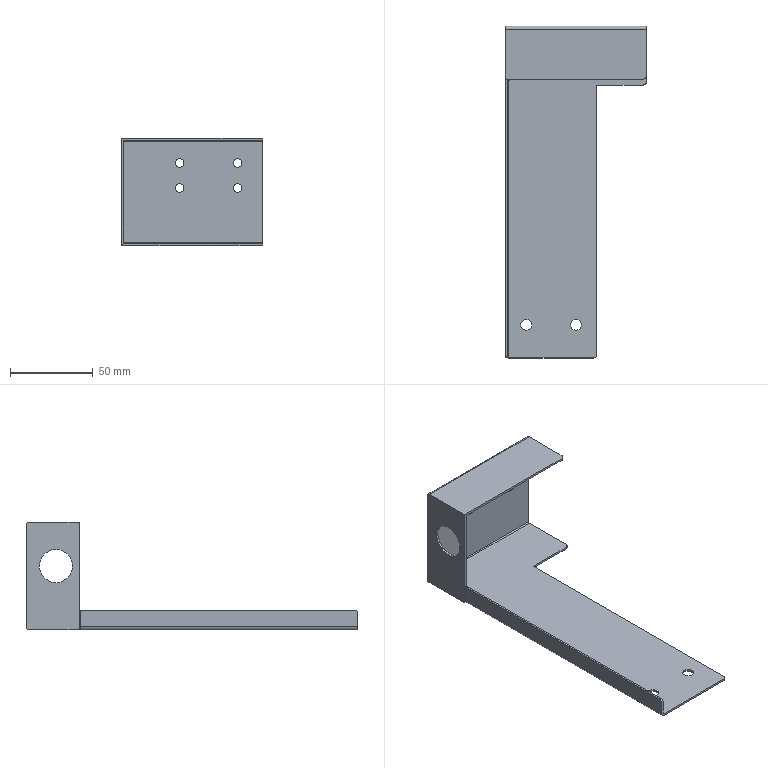Part | 1 solid | 50 faces | box 85 x 200 x 65 mm | volume 27815 mm3 | plane 26 | cylinder 24 | commonest cylinder face diameters 5.2 x8 4 x4 6.5 x4 1.473 x3 3.873 x3 20 x2
STEP:
#1=CARTESIAN_POINT('',(-26.3,82.,47.3));
#2=VERTEX_POINT('',#1);
#3=CARTESIAN_POINT('',(-26.3,82.,27.3));
#4=VERTEX_POINT('',#3);
#5=CARTESIAN_POINT('',(-26.3,82.,37.3));
#6=DIRECTION('',(1.,0.,0.));
#7=DIRECTION('',(0.,0.,-1.));
#8=AXIS2_PLACEMENT_3D('',#5,#6,#7);
#9=CIRCLE('',#8,10.);
#10=EDGE_CURVE('',#2,#4,#9,.T.);
#11=ORIENTED_EDGE('',*,*,#10,.T.);
#12=CARTESIAN_POINT('',(-27.5,82.,27.3));
#13=VERTEX_POINT('',#12);
#14=CARTESIAN_POINT('',(57.5,82.,27.3));
#15=DIRECTION('',(-1.,0.,0.));
#16=VECTOR('',#15,1000.);
#17=LINE('',#14,#16);
#18=EDGE_CURVE('',#4,#13,#17,.T.);
#19=ORIENTED_EDGE('',*,*,#18,.T.);
#20=CARTESIAN_POINT('',(-27.5,82.,47.3));
#21=VERTEX_POINT('',#20);
#22=CARTESIAN_POINT('',(-27.5,82.,37.3));
#23=DIRECTION('',(-1.,0.,0.));
#24=DIRECTION('',(0.,0.,1.));
#25=AXIS2_PLACEMENT_3D('',#22,#23,#24);
#26=CIRCLE('',#25,10.);
#27=EDGE_CURVE('',#13,#21,#26,.T.);
#28=ORIENTED_EDGE('',*,*,#27,.T.);
#29=CARTESIAN_POINT('',(57.5,82.,47.3));
#30=DIRECTION('',(-1.,0.,0.));
#31=VECTOR('',#30,1000.);
#32=LINE('',#29,#31);
#33=EDGE_CURVE('',#2,#21,#32,.T.);
#34=ORIENTED_EDGE('',*,*,#33,.F.);
#35=EDGE_LOOP('',(#11,#19,#28,#34));
#36=FACE_OUTER_BOUND('',#35,.T.);
#37=CARTESIAN_POINT('',(57.5,82.,37.3));
#38=DIRECTION('',(-1.,0.,0.));
#39=DIRECTION('',(0.,0.,1.));
#40=AXIS2_PLACEMENT_3D('',#37,#38,#39);
#41=CYLINDRICAL_SURFACE('',#40,10.);
#42=ADVANCED_FACE('',(#36),#41,.F.);
#43=CARTESIAN_POINT('',(42.5,98.8,46.2));
#44=VERTEX_POINT('',#43);
#45=CARTESIAN_POINT('',(42.5,98.8,51.4));
#46=VERTEX_POINT('',#45);
#47=CARTESIAN_POINT('',(42.5,98.8,48.8));
#48=DIRECTION('',(0.,1.,0.));
#49=DIRECTION('',(0.,0.,1.));
#50=AXIS2_PLACEMENT_3D('',#47,#48,#49);
#51=CIRCLE('',#50,2.6);
#52=EDGE_CURVE('',#44,#46,#51,.T.);
#53=ORIENTED_EDGE('',*,*,#52,.F.);
#54=CARTESIAN_POINT('',(42.5,100.,46.2));
#55=VERTEX_POINT('',#54);
#56=CARTESIAN_POINT('',(42.5,90.,46.2));
#57=DIRECTION('',(0.,1.,0.));
#58=VECTOR('',#57,1000.);
#59=LINE('',#56,#58);
#60=EDGE_CURVE('',#44,#55,#59,.T.);
#61=ORIENTED_EDGE('',*,*,#60,.T.);
#62=CARTESIAN_POINT('',(42.5,100.,51.4));
#63=VERTEX_POINT('',#62);
#64=CARTESIAN_POINT('',(42.5,100.,48.8));
#65=DIRECTION('',(0.,1.,0.));
#66=DIRECTION('',(0.,0.,1.));
#67=AXIS2_PLACEMENT_3D('',#64,#65,#66);
#68=CIRCLE('',#67,2.6);
#69=EDGE_CURVE('',#55,#63,#68,.T.);
#70=ORIENTED_EDGE('',*,*,#69,.T.);
#71=CARTESIAN_POINT('',(42.5,90.,51.4));
#72=DIRECTION('',(0.,1.,0.));
#73=VECTOR('',#72,1000.);
#74=LINE('',#71,#73);
#75=EDGE_CURVE('',#46,#63,#74,.T.);
#76=ORIENTED_EDGE('',*,*,#75,.F.);
#77=EDGE_LOOP('',(#53,#61,#70,#76));
#78=FACE_OUTER_BOUND('',#77,.T.);
#79=CARTESIAN_POINT('',(42.5,90.,48.8));
#80=DIRECTION('',(0.,1.,0.));
#81=DIRECTION('',(0.,0.,1.));
#82=AXIS2_PLACEMENT_3D('',#79,#80,#81);
#83=CYLINDRICAL_SURFACE('',#82,2.6);
#84=ADVANCED_FACE('',(#78),#83,.F.);
#85=CARTESIAN_POINT('',(7.5,98.8,46.2));
#86=VERTEX_POINT('',#85);
#87=CARTESIAN_POINT('',(7.5,98.8,51.4));
#88=VERTEX_POINT('',#87);
#89=CARTESIAN_POINT('',(7.5,98.8,48.8));
#90=DIRECTION('',(0.,1.,0.));
#91=DIRECTION('',(0.,0.,1.));
#92=AXIS2_PLACEMENT_3D('',#89,#90,#91);
#93=CIRCLE('',#92,2.6);
#94=EDGE_CURVE('',#86,#88,#93,.T.);
#95=ORIENTED_EDGE('',*,*,#94,.F.);
#96=CARTESIAN_POINT('',(7.5,100.,46.2));
#97=VERTEX_POINT('',#96);
#98=CARTESIAN_POINT('',(7.5,90.,46.2));
#99=DIRECTION('',(0.,1.,0.));
#100=VECTOR('',#99,1000.);
#101=LINE('',#98,#100);
#102=EDGE_CURVE('',#86,#97,#101,.T.);
#103=ORIENTED_EDGE('',*,*,#102,.T.);
#104=CARTESIAN_POINT('',(7.5,100.,51.4));
#105=VERTEX_POINT('',#104);
#106=CARTESIAN_POINT('',(7.5,100.,48.8));
#107=DIRECTION('',(0.,1.,0.));
#108=DIRECTION('',(0.,0.,1.));
#109=AXIS2_PLACEMENT_3D('',#106,#107,#108);
#110=CIRCLE('',#109,2.6);
#111=EDGE_CURVE('',#97,#105,#110,.T.);
#112=ORIENTED_EDGE('',*,*,#111,.T.);
#113=CARTESIAN_POINT('',(7.5,90.,51.4));
#114=DIRECTION('',(0.,1.,0.));
#115=VECTOR('',#114,1000.);
#116=LINE('',#113,#115);
#117=EDGE_CURVE('',#88,#105,#116,.T.);
#118=ORIENTED_EDGE('',*,*,#117,.F.);
#119=EDGE_LOOP('',(#95,#103,#112,#118));
#120=FACE_OUTER_BOUND('',#119,.T.);
#121=CARTESIAN_POINT('',(7.5,90.,48.8));
#122=DIRECTION('',(0.,1.,0.));
#123=DIRECTION('',(0.,0.,1.));
#124=AXIS2_PLACEMENT_3D('',#121,#122,#123);
#125=CYLINDRICAL_SURFACE('',#124,2.6);
#126=ADVANCED_FACE('',(#120),#125,.F.);
#127=CARTESIAN_POINT('',(7.5,98.8,31.2));
#128=VERTEX_POINT('',#127);
#129=CARTESIAN_POINT('',(7.5,98.8,36.4));
#130=VERTEX_POINT('',#129);
#131=CARTESIAN_POINT('',(7.5,98.8,33.8));
#132=DIRECTION('',(0.,1.,0.));
#133=DIRECTION('',(0.,0.,1.));
#134=AXIS2_PLACEMENT_3D('',#131,#132,#133);
#135=CIRCLE('',#134,2.6);
#136=EDGE_CURVE('',#128,#130,#135,.T.);
#137=ORIENTED_EDGE('',*,*,#136,.F.);
#138=CARTESIAN_POINT('',(7.5,100.,31.2));
#139=VERTEX_POINT('',#138);
#140=CARTESIAN_POINT('',(7.5,90.,31.2));
#141=DIRECTION('',(0.,1.,0.));
#142=VECTOR('',#141,1000.);
#143=LINE('',#140,#142);
#144=EDGE_CURVE('',#128,#139,#143,.T.);
#145=ORIENTED_EDGE('',*,*,#144,.T.);
#146=CARTESIAN_POINT('',(7.5,100.,36.4));
#147=VERTEX_POINT('',#146);
#148=CARTESIAN_POINT('',(7.5,100.,33.8));
#149=DIRECTION('',(0.,1.,0.));
#150=DIRECTION('',(0.,0.,1.));
#151=AXIS2_PLACEMENT_3D('',#148,#149,#150);
#152=CIRCLE('',#151,2.6);
#153=EDGE_CURVE('',#139,#147,#152,.T.);
#154=ORIENTED_EDGE('',*,*,#153,.T.);
#155=CARTESIAN_POINT('',(7.5,90.,36.4));
#156=DIRECTION('',(0.,1.,0.));
#157=VECTOR('',#156,1000.);
#158=LINE('',#155,#157);
#159=EDGE_CURVE('',#130,#147,#158,.T.);
#160=ORIENTED_EDGE('',*,*,#159,.F.);
#161=EDGE_LOOP('',(#137,#145,#154,#160));
#162=FACE_OUTER_BOUND('',#161,.T.);
#163=CARTESIAN_POINT('',(7.5,90.,33.8));
#164=DIRECTION('',(0.,1.,0.));
#165=DIRECTION('',(0.,0.,1.));
#166=AXIS2_PLACEMENT_3D('',#163,#164,#165);
#167=CYLINDRICAL_SURFACE('',#166,2.6);
#168=ADVANCED_FACE('',(#162),#167,.F.);
#169=CARTESIAN_POINT('',(42.5,98.8,31.2));
#170=VERTEX_POINT('',#169);
#171=CARTESIAN_POINT('',(42.5,98.8,36.4));
#172=VERTEX_POINT('',#171);
#173=CARTESIAN_POINT('',(42.5,98.8,33.8));
#174=DIRECTION('',(0.,1.,0.));
#175=DIRECTION('',(0.,0.,1.));
#176=AXIS2_PLACEMENT_3D('',#173,#174,#175);
#177=CIRCLE('',#176,2.6);
#178=EDGE_CURVE('',#170,#172,#177,.T.);
#179=ORIENTED_EDGE('',*,*,#178,.F.);
#180=CARTESIAN_POINT('',(42.5,100.,31.2));
#181=VERTEX_POINT('',#180);
#182=CARTESIAN_POINT('',(42.5,90.,31.2));
#183=DIRECTION('',(0.,1.,0.));
#184=VECTOR('',#183,1000.);
#185=LINE('',#182,#184);
#186=EDGE_CURVE('',#170,#181,#185,.T.);
#187=ORIENTED_EDGE('',*,*,#186,.T.);
#188=CARTESIAN_POINT('',(42.5,100.,36.4));
#189=VERTEX_POINT('',#188);
#190=CARTESIAN_POINT('',(42.5,100.,33.8));
#191=DIRECTION('',(0.,1.,0.));
#192=DIRECTION('',(0.,0.,1.));
#193=AXIS2_PLACEMENT_3D('',#190,#191,#192);
#194=CIRCLE('',#193,2.6);
#195=EDGE_CURVE('',#181,#189,#194,.T.);
#196=ORIENTED_EDGE('',*,*,#195,.T.);
#197=CARTESIAN_POINT('',(42.5,90.,36.4));
#198=DIRECTION('',(0.,1.,0.));
#199=VECTOR('',#198,1000.);
#200=LINE('',#197,#199);
#201=EDGE_CURVE('',#172,#189,#200,.T.);
#202=ORIENTED_EDGE('',*,*,#201,.F.);
#203=EDGE_LOOP('',(#179,#187,#196,#202));
#204=FACE_OUTER_BOUND('',#203,.T.);
#205=CARTESIAN_POINT('',(42.5,90.,33.8));
#206=DIRECTION('',(0.,1.,0.));
#207=DIRECTION('',(0.,0.,1.));
#208=AXIS2_PLACEMENT_3D('',#205,#206,#207);
#209=CYLINDRICAL_SURFACE('',#208,2.6);
#210=ADVANCED_FACE('',(#204),#209,.F.);
#211=CARTESIAN_POINT('',(18.25,-80.,0.));
#212=VERTEX_POINT('',#211);
#213=CARTESIAN_POINT('',(11.75,-80.,0.));
#214=VERTEX_POINT('',#213);
#215=CARTESIAN_POINT('',(15.,-80.,0.));
#216=DIRECTION('',(0.,0.,-1.));
#217=DIRECTION('',(-1.,0.,0.));
#218=AXIS2_PLACEMENT_3D('',#215,#216,#217);
#219=CIRCLE('',#218,3.25);
#220=EDGE_CURVE('',#212,#214,#219,.T.);
#221=ORIENTED_EDGE('',*,*,#220,.F.);
#222=CARTESIAN_POINT('',(18.25,-80.,-1.2));
#223=VERTEX_POINT('',#222);
#224=CARTESIAN_POINT('',(18.25,-80.,8.8));
#225=DIRECTION('',(0.,0.,-1.));
#226=VECTOR('',#225,1000.);
#227=LINE('',#224,#226);
#228=EDGE_CURVE('',#212,#223,#227,.T.);
#229=ORIENTED_EDGE('',*,*,#228,.T.);
#230=CARTESIAN_POINT('',(11.75,-80.,-1.2));
#231=VERTEX_POINT('',#230);
#232=CARTESIAN_POINT('',(15.,-80.,-1.2));
#233=DIRECTION('',(0.,0.,-1.));
#234=DIRECTION('',(-1.,0.,0.));
#235=AXIS2_PLACEMENT_3D('',#232,#233,#234);
#236=CIRCLE('',#235,3.25);
#237=EDGE_CURVE('',#223,#231,#236,.T.);
#238=ORIENTED_EDGE('',*,*,#237,.T.);
#239=CARTESIAN_POINT('',(11.75,-80.,8.8));
#240=DIRECTION('',(0.,0.,-1.));
#241=VECTOR('',#240,1000.);
#242=LINE('',#239,#241);
#243=EDGE_CURVE('',#214,#231,#242,.T.);
#244=ORIENTED_EDGE('',*,*,#243,.F.);
#245=EDGE_LOOP('',(#221,#229,#238,#244));
#246=FACE_OUTER_BOUND('',#245,.T.);
#247=CARTESIAN_POINT('',(15.,-80.,8.8));
#248=DIRECTION('',(0.,0.,-1.));
#249=DIRECTION('',(-1.,0.,0.));
#250=AXIS2_PLACEMENT_3D('',#247,#248,#249);
#251=CYLINDRICAL_SURFACE('',#250,3.25);
#252=ADVANCED_FACE('',(#246),#251,.F.);
#253=CARTESIAN_POINT('',(-11.75,-80.,0.));
#254=VERTEX_POINT('',#253);
#255=CARTESIAN_POINT('',(-18.25,-80.,0.));
#256=VERTEX_POINT('',#255);
#257=CARTESIAN_POINT('',(-15.,-80.,0.));
#258=DIRECTION('',(0.,0.,-1.));
#259=DIRECTION('',(-1.,0.,0.));
#260=AXIS2_PLACEMENT_3D('',#257,#258,#259);
#261=CIRCLE('',#260,3.25);
#262=EDGE_CURVE('',#254,#256,#261,.T.);
#263=ORIENTED_EDGE('',*,*,#262,.F.);
#264=CARTESIAN_POINT('',(-11.75,-80.,-1.2));
#265=VERTEX_POINT('',#264);
#266=CARTESIAN_POINT('',(-11.75,-80.,8.8));
#267=DIRECTION('',(0.,0.,-1.));
#268=VECTOR('',#267,1000.);
#269=LINE('',#266,#268);
#270=EDGE_CURVE('',#254,#265,#269,.T.);
#271=ORIENTED_EDGE('',*,*,#270,.T.);
#272=CARTESIAN_POINT('',(-18.25,-80.,-1.2));
#273=VERTEX_POINT('',#272);
#274=CARTESIAN_POINT('',(-15.,-80.,-1.2));
#275=DIRECTION('',(0.,0.,-1.));
#276=DIRECTION('',(-1.,0.,0.));
#277=AXIS2_PLACEMENT_3D('',#274,#275,#276);
#278=CIRCLE('',#277,3.25);
#279=EDGE_CURVE('',#265,#273,#278,.T.);
#280=ORIENTED_EDGE('',*,*,#279,.T.);
#281=CARTESIAN_POINT('',(-18.25,-80.,8.8));
#282=DIRECTION('',(0.,0.,-1.));
#283=VECTOR('',#282,1000.);
#284=LINE('',#281,#283);
#285=EDGE_CURVE('',#256,#273,#284,.T.);
#286=ORIENTED_EDGE('',*,*,#285,.F.);
#287=EDGE_LOOP('',(#263,#271,#280,#286));
#288=FACE_OUTER_BOUND('',#287,.T.);
#289=CARTESIAN_POINT('',(-15.,-80.,8.8));
#290=DIRECTION('',(0.,0.,-1.));
#291=DIRECTION('',(-1.,0.,0.));
#292=AXIS2_PLACEMENT_3D('',#289,#290,#291);
#293=CYLINDRICAL_SURFACE('',#292,3.25);
#294=ADVANCED_FACE('',(#288),#293,.F.);
#295=CARTESIAN_POINT('',(27.5,64.5,-1.2));
#296=VERTEX_POINT('',#295);
#297=CARTESIAN_POINT('',(27.5,-98.,-1.2));
#298=VERTEX_POINT('',#297);
#299=CARTESIAN_POINT('',(27.5,-100.,-1.2));
#300=DIRECTION('',(0.,-1.,0.));
#301=VECTOR('',#300,1000.);
#302=LINE('',#299,#301);
#303=EDGE_CURVE('',#296,#298,#302,.T.);
#304=ORIENTED_EDGE('',*,*,#303,.T.);
#305=CARTESIAN_POINT('',(25.5,-100.,-1.2));
#306=VERTEX_POINT('',#305);
#307=CARTESIAN_POINT('',(25.5,-98.,-1.2));
#308=DIRECTION('',(0.,0.,-1.));
#309=DIRECTION('',(-1.,0.,0.));
#310=AXIS2_PLACEMENT_3D('',#307,#308,#309);
#311=CIRCLE('',#310,2.);
#312=EDGE_CURVE('',#298,#306,#311,.T.);
#313=ORIENTED_EDGE('',*,*,#312,.T.);
#314=CARTESIAN_POINT('',(-25.563,-100.,-1.2));
#315=VERTEX_POINT('',#314);
#316=CARTESIAN_POINT('',(-27.5,-100.,-1.2));
#317=DIRECTION('',(1.,0.,0.));
#318=VECTOR('',#317,1000.);
#319=LINE('',#316,#318);
#320=EDGE_CURVE('',#315,#306,#319,.T.);
#321=ORIENTED_EDGE('',*,*,#320,.F.);
#322=CARTESIAN_POINT('',(-25.563,67.5,-1.2));
#323=VERTEX_POINT('',#322);
#324=CARTESIAN_POINT('',(-25.563,-100.,-1.2));
#325=DIRECTION('',(0.,1.,0.));
#326=VECTOR('',#325,1000.);
#327=LINE('',#324,#326);
#328=EDGE_CURVE('',#315,#323,#327,.T.);
#329=ORIENTED_EDGE('',*,*,#328,.T.);
#330=CARTESIAN_POINT('',(-24.963,67.5,-1.2));
#331=VERTEX_POINT('',#330);
#332=CARTESIAN_POINT('',(0.,67.5,-1.2));
#333=DIRECTION('',(1.,0.,0.));
#334=VECTOR('',#333,1000.);
#335=LINE('',#332,#334);
#336=EDGE_CURVE('',#323,#331,#335,.T.);
#337=ORIENTED_EDGE('',*,*,#336,.T.);
#338=CARTESIAN_POINT('',(-24.963,68.1,-1.2));
#339=VERTEX_POINT('',#338);
#340=CARTESIAN_POINT('',(-24.963,0.,-1.2));
#341=DIRECTION('',(0.,1.,0.));
#342=VECTOR('',#341,1000.);
#343=LINE('',#340,#342);
#344=EDGE_CURVE('',#331,#339,#343,.T.);
#345=ORIENTED_EDGE('',*,*,#344,.T.);
#346=CARTESIAN_POINT('',(-26.3,68.1,-1.2));
#347=VERTEX_POINT('',#346);
#348=CARTESIAN_POINT('',(0.,68.1,-1.2));
#349=DIRECTION('',(-1.,0.,0.));
#350=VECTOR('',#349,1000.);
#351=LINE('',#348,#350);
#352=EDGE_CURVE('',#339,#347,#351,.T.);
#353=ORIENTED_EDGE('',*,*,#352,.T.);
#354=CARTESIAN_POINT('',(-26.3,68.,-1.2));
#355=VERTEX_POINT('',#354);
#356=CARTESIAN_POINT('',(-26.3,68.,-1.2));
#357=DIRECTION('',(0.,-1.,0.));
#358=VECTOR('',#357,1000.);
#359=LINE('',#356,#358);
#360=EDGE_CURVE('',#347,#355,#359,.T.);
#361=ORIENTED_EDGE('',*,*,#360,.T.);
#362=CARTESIAN_POINT('',(-27.5,68.,-1.2));
#363=VERTEX_POINT('',#362);
#364=CARTESIAN_POINT('',(-26.3,68.,-1.2));
#365=DIRECTION('',(-1.,0.,0.));
#366=VECTOR('',#365,1000.);
#367=LINE('',#364,#366);
#368=EDGE_CURVE('',#355,#363,#367,.T.);
#369=ORIENTED_EDGE('',*,*,#368,.T.);
#370=CARTESIAN_POINT('',(-27.5,98.063,-1.2));
#371=VERTEX_POINT('',#370);
#372=CARTESIAN_POINT('',(-27.5,-100.,-1.2));
#373=DIRECTION('',(0.,-1.,0.));
#374=VECTOR('',#373,1000.);
#375=LINE('',#372,#374);
#376=EDGE_CURVE('',#371,#363,#375,.T.);
#377=ORIENTED_EDGE('',*,*,#376,.F.);
#378=CARTESIAN_POINT('',(57.5,98.063,-1.2));
#379=VERTEX_POINT('',#378);
#380=CARTESIAN_POINT('',(-27.5,98.063,-1.2));
#381=DIRECTION('',(1.,0.,0.));
#382=VECTOR('',#381,1000.);
#383=LINE('',#380,#382);
#384=EDGE_CURVE('',#371,#379,#383,.T.);
#385=ORIENTED_EDGE('',*,*,#384,.T.);
#386=CARTESIAN_POINT('',(57.5,66.5,-1.2));
#387=VERTEX_POINT('',#386);
#388=CARTESIAN_POINT('',(57.5,-100.,-1.2));
#389=DIRECTION('',(0.,1.,0.));
#390=VECTOR('',#389,1000.);
#391=LINE('',#388,#390);
#392=EDGE_CURVE('',#387,#379,#391,.T.);
#393=ORIENTED_EDGE('',*,*,#392,.F.);
#394=CARTESIAN_POINT('',(55.5,64.5,-1.2));
#395=VERTEX_POINT('',#394);
#396=CARTESIAN_POINT('',(55.5,66.5,-1.2));
#397=DIRECTION('',(0.,0.,-1.));
#398=DIRECTION('',(-1.,0.,0.));
#399=AXIS2_PLACEMENT_3D('',#396,#397,#398);
#400=CIRCLE('',#399,2.);
#401=EDGE_CURVE('',#387,#395,#400,.T.);
#402=ORIENTED_EDGE('',*,*,#401,.T.);
#403=CARTESIAN_POINT('',(57.5,64.5,-1.2));
#404=DIRECTION('',(-1.,0.,0.));
#405=VECTOR('',#404,1000.);
#406=LINE('',#403,#405);
#407=EDGE_CURVE('',#395,#296,#406,.T.);
#408=ORIENTED_EDGE('',*,*,#407,.T.);
#409=EDGE_LOOP('',(#304,#313,#321,#329,#337,#345,#353,#361,#369,#377,#385,#393,#402,#408));
#410=FACE_OUTER_BOUND('',#409,.T.);
#411=CARTESIAN_POINT('',(15.,-80.,-1.2));
#412=DIRECTION('',(0.,0.,-1.));
#413=DIRECTION('',(-1.,0.,0.));
#414=AXIS2_PLACEMENT_3D('',#411,#412,#413);
#415=CIRCLE('',#414,3.25);
#416=EDGE_CURVE('',#231,#223,#415,.T.);
#417=ORIENTED_EDGE('',*,*,#416,.F.);
#418=ORIENTED_EDGE('',*,*,#237,.F.);
#419=EDGE_LOOP('',(#417,#418));
#420=FACE_BOUND('',#419,.T.);
#421=CARTESIAN_POINT('',(-15.,-80.,-1.2));
#422=DIRECTION('',(0.,0.,-1.));
#423=DIRECTION('',(-1.,0.,0.));
#424=AXIS2_PLACEMENT_3D('',#421,#422,#423);
#425=CIRCLE('',#424,3.25);
#426=EDGE_CURVE('',#273,#265,#425,.T.);
#427=ORIENTED_EDGE('',*,*,#426,.F.);
#428=ORIENTED_EDGE('',*,*,#279,.F.);
#429=EDGE_LOOP('',(#427,#428));
#430=FACE_BOUND('',#429,.T.);
#431=CARTESIAN_POINT('',(0.,0.,-1.2));
#432=DIRECTION('',(0.,0.,-1.));
#433=DIRECTION('',(-1.,0.,0.));
#434=AXIS2_PLACEMENT_3D('',#431,#432,#433);
#435=PLANE('',#434);
#436=ADVANCED_FACE('',(#410,#420,#430),#435,.T.);
#437=CARTESIAN_POINT('',(-15.,-80.,0.));
#438=DIRECTION('',(0.,0.,-1.));
#439=DIRECTION('',(-1.,0.,0.));
#440=AXIS2_PLACEMENT_3D('',#437,#438,#439);
#441=CIRCLE('',#440,3.25);
#442=EDGE_CURVE('',#256,#254,#441,.T.);
#443=ORIENTED_EDGE('',*,*,#442,.T.);
#444=ORIENTED_EDGE('',*,*,#262,.T.);
#445=EDGE_LOOP('',(#443,#444));
#446=FACE_BOUND('',#445,.T.);
#447=CARTESIAN_POINT('',(15.,-80.,0.));
#448=DIRECTION('',(0.,0.,-1.));
#449=DIRECTION('',(-1.,0.,0.));
#450=AXIS2_PLACEMENT_3D('',#447,#448,#449);
#451=CIRCLE('',#450,3.25);
#452=EDGE_CURVE('',#214,#212,#451,.T.);
#453=ORIENTED_EDGE('',*,*,#452,.T.);
#454=ORIENTED_EDGE('',*,*,#220,.T.);
#455=EDGE_LOOP('',(#453,#454));
#456=FACE_BOUND('',#455,.T.);
#457=CARTESIAN_POINT('',(-25.563,-100.,0.));
#458=VERTEX_POINT('',#457);
#459=CARTESIAN_POINT('',(25.5,-100.,0.));
#460=VERTEX_POINT('',#459);
#461=CARTESIAN_POINT('',(-27.5,-100.,0.));
#462=DIRECTION('',(1.,0.,0.));
#463=VECTOR('',#462,1000.);
#464=LINE('',#461,#463);
#465=EDGE_CURVE('',#458,#460,#464,.T.);
#466=ORIENTED_EDGE('',*,*,#465,.T.);
#467=CARTESIAN_POINT('',(27.5,-98.,0.));
#468=VERTEX_POINT('',#467);
#469=CARTESIAN_POINT('',(25.5,-98.,0.));
#470=DIRECTION('',(0.,0.,1.));
#471=DIRECTION('',(-1.,0.,0.));
#472=AXIS2_PLACEMENT_3D('',#469,#470,#471);
#473=CIRCLE('',#472,2.);
#474=EDGE_CURVE('',#460,#468,#473,.T.);
#475=ORIENTED_EDGE('',*,*,#474,.T.);
#476=CARTESIAN_POINT('',(27.5,64.5,0.));
#477=VERTEX_POINT('',#476);
#478=CARTESIAN_POINT('',(27.5,-100.,0.));
#479=DIRECTION('',(0.,-1.,0.));
#480=VECTOR('',#479,1000.);
#481=LINE('',#478,#480);
#482=EDGE_CURVE('',#477,#468,#481,.T.);
#483=ORIENTED_EDGE('',*,*,#482,.F.);
#484=CARTESIAN_POINT('',(55.5,64.5,0.));
#485=VERTEX_POINT('',#484);
#486=CARTESIAN_POINT('',(57.5,64.5,0.));
#487=DIRECTION('',(-1.,0.,0.));
#488=VECTOR('',#487,1000.);
#489=LINE('',#486,#488);
#490=EDGE_CURVE('',#485,#477,#489,.T.);
#491=ORIENTED_EDGE('',*,*,#490,.F.);
#492=CARTESIAN_POINT('',(57.5,66.5,0.));
#493=VERTEX_POINT('',#492);
#494=CARTESIAN_POINT('',(55.5,66.5,0.));
#495=DIRECTION('',(0.,0.,1.));
#496=DIRECTION('',(-1.,0.,0.));
#497=AXIS2_PLACEMENT_3D('',#494,#495,#496);
#498=CIRCLE('',#497,2.);
#499=EDGE_CURVE('',#485,#493,#498,.T.);
#500=ORIENTED_EDGE('',*,*,#499,.T.);
#501=CARTESIAN_POINT('',(57.5,98.063,0.));
#502=VERTEX_POINT('',#501);
#503=CARTESIAN_POINT('',(57.5,-100.,0.));
#504=DIRECTION('',(0.,1.,0.));
#505=VECTOR('',#504,1000.);
#506=LINE('',#503,#505);
#507=EDGE_CURVE('',#493,#502,#506,.T.);
#508=ORIENTED_EDGE('',*,*,#507,.T.);
#509=CARTESIAN_POINT('',(-26.3,98.063,0.));
#510=VERTEX_POINT('',#509);
#511=CARTESIAN_POINT('',(-27.5,98.063,0.));
#512=DIRECTION('',(1.,0.,0.));
#513=VECTOR('',#512,1000.);
#514=LINE('',#511,#513);
#515=EDGE_CURVE('',#510,#502,#514,.T.);
#516=ORIENTED_EDGE('',*,*,#515,.F.);
#517=CARTESIAN_POINT('',(-26.3,68.1,0.));
#518=VERTEX_POINT('',#517);
#519=CARTESIAN_POINT('',(-26.3,0.,0.));
#520=DIRECTION('',(0.,-1.,0.));
#521=VECTOR('',#520,1000.);
#522=LINE('',#519,#521);
#523=EDGE_CURVE('',#510,#518,#522,.T.);
#524=ORIENTED_EDGE('',*,*,#523,.T.);
#525=CARTESIAN_POINT('',(-24.963,68.1,0.));
#526=VERTEX_POINT('',#525);
#527=CARTESIAN_POINT('',(-24.963,68.1,0.));
#528=DIRECTION('',(-1.,0.,0.));
#529=VECTOR('',#528,1000.);
#530=LINE('',#527,#529);
#531=EDGE_CURVE('',#526,#518,#530,.T.);
#532=ORIENTED_EDGE('',*,*,#531,.F.);
#533=CARTESIAN_POINT('',(-24.963,67.5,0.));
#534=VERTEX_POINT('',#533);
#535=CARTESIAN_POINT('',(-24.963,67.5,0.));
#536=DIRECTION('',(0.,1.,0.));
#537=VECTOR('',#536,1000.);
#538=LINE('',#535,#537);
#539=EDGE_CURVE('',#534,#526,#538,.T.);
#540=ORIENTED_EDGE('',*,*,#539,.F.);
#541=CARTESIAN_POINT('',(-25.563,67.5,0.));
#542=VERTEX_POINT('',#541);
#543=CARTESIAN_POINT('',(-25.563,67.5,0.));
#544=DIRECTION('',(1.,0.,0.));
#545=VECTOR('',#544,1000.);
#546=LINE('',#543,#545);
#547=EDGE_CURVE('',#542,#534,#546,.T.);
#548=ORIENTED_EDGE('',*,*,#547,.F.);
#549=CARTESIAN_POINT('',(-25.563,-100.,0.));
#550=DIRECTION('',(0.,1.,0.));
#551=VECTOR('',#550,1000.);
#552=LINE('',#549,#551);
#553=EDGE_CURVE('',#458,#542,#552,.T.);
#554=ORIENTED_EDGE('',*,*,#553,.F.);
#555=EDGE_LOOP('',(#466,#475,#483,#491,#500,#508,#516,#524,#532,#540,#548,#554));
#556=FACE_OUTER_BOUND('',#555,.T.);
#557=CARTESIAN_POINT('',(0.,0.,0.));
#558=DIRECTION('',(0.,0.,-1.));
#559=DIRECTION('',(-1.,0.,0.));
#560=AXIS2_PLACEMENT_3D('',#557,#558,#559);
#561=PLANE('',#560);
#562=ADVANCED_FACE('',(#446,#456,#556),#561,.F.);
#563=ORIENTED_EDGE('',*,*,#320,.T.);
#564=CARTESIAN_POINT('',(25.5,-100.,0.));
#565=DIRECTION('',(0.,0.,1.));
#566=VECTOR('',#565,1000.);
#567=LINE('',#564,#566);
#568=EDGE_CURVE('',#306,#460,#567,.T.);
#569=ORIENTED_EDGE('',*,*,#568,.T.);
#570=ORIENTED_EDGE('',*,*,#465,.F.);
#571=CARTESIAN_POINT('',(-25.563,-100.,0.));
#572=DIRECTION('',(0.,0.,-1.));
#573=VECTOR('',#572,1000.);
#574=LINE('',#571,#573);
#575=EDGE_CURVE('',#458,#315,#574,.T.);
#576=ORIENTED_EDGE('',*,*,#575,.T.);
#577=EDGE_LOOP('',(#563,#569,#570,#576));
#578=FACE_OUTER_BOUND('',#577,.T.);
#579=CARTESIAN_POINT('',(-27.5,-100.,-1.2));
#580=DIRECTION('',(0.,-1.,0.));
#581=DIRECTION('',(0.,0.,-1.));
#582=AXIS2_PLACEMENT_3D('',#579,#580,#581);
#583=PLANE('',#582);
#584=ADVANCED_FACE('',(#578),#583,.T.);
#585=CARTESIAN_POINT('',(57.5,100.,0.7366));
#586=VERTEX_POINT('',#585);
#587=CARTESIAN_POINT('',(-27.5,100.,0.7366));
#588=VERTEX_POINT('',#587);
#589=CARTESIAN_POINT('',(-27.5,100.,0.7366));
#590=DIRECTION('',(-1.,0.,0.));
#591=VECTOR('',#590,1000.);
#592=LINE('',#589,#591);
#593=EDGE_CURVE('',#586,#588,#592,.T.);
#594=ORIENTED_EDGE('',*,*,#593,.T.);
#595=CARTESIAN_POINT('',(-27.5,100.,61.863));
#596=VERTEX_POINT('',#595);
#597=CARTESIAN_POINT('',(-27.5,100.,0.));
#598=DIRECTION('',(0.,0.,-1.));
#599=VECTOR('',#598,1000.);
#600=LINE('',#597,#599);
#601=EDGE_CURVE('',#596,#588,#600,.T.);
#602=ORIENTED_EDGE('',*,*,#601,.F.);
#603=CARTESIAN_POINT('',(57.5,100.,61.863));
#604=VERTEX_POINT('',#603);
#605=CARTESIAN_POINT('',(-27.5,100.,61.863));
#606=DIRECTION('',(1.,0.,0.));
#607=VECTOR('',#606,1000.);
#608=LINE('',#605,#607);
#609=EDGE_CURVE('',#596,#604,#608,.T.);
#610=ORIENTED_EDGE('',*,*,#609,.T.);
#611=CARTESIAN_POINT('',(57.5,100.,63.8));
#612=DIRECTION('',(0.,0.,1.));
#613=VECTOR('',#612,1000.);
#614=LINE('',#611,#613);
#615=EDGE_CURVE('',#586,#604,#614,.T.);
#616=ORIENTED_EDGE('',*,*,#615,.F.);
#617=EDGE_LOOP('',(#594,#602,#610,#616));
#618=FACE_OUTER_BOUND('',#617,.T.);
#619=CARTESIAN_POINT('',(42.5,100.,48.8));
#620=DIRECTION('',(0.,1.,0.));
#621=DIRECTION('',(0.,0.,1.));
#622=AXIS2_PLACEMENT_3D('',#619,#620,#621);
#623=CIRCLE('',#622,2.6);
#624=EDGE_CURVE('',#63,#55,#623,.T.);
#625=ORIENTED_EDGE('',*,*,#624,.F.);
#626=ORIENTED_EDGE('',*,*,#69,.F.);
#627=EDGE_LOOP('',(#625,#626));
#628=FACE_BOUND('',#627,.T.);
#629=CARTESIAN_POINT('',(7.5,100.,48.8));
#630=DIRECTION('',(0.,1.,0.));
#631=DIRECTION('',(0.,0.,1.));
#632=AXIS2_PLACEMENT_3D('',#629,#630,#631);
#633=CIRCLE('',#632,2.6);
#634=EDGE_CURVE('',#105,#97,#633,.T.);
#635=ORIENTED_EDGE('',*,*,#634,.F.);
#636=ORIENTED_EDGE('',*,*,#111,.F.);
#637=EDGE_LOOP('',(#635,#636));
#638=FACE_BOUND('',#637,.T.);
#639=CARTESIAN_POINT('',(7.5,100.,33.8));
#640=DIRECTION('',(0.,1.,0.));
#641=DIRECTION('',(0.,0.,1.));
#642=AXIS2_PLACEMENT_3D('',#639,#640,#641);
#643=CIRCLE('',#642,2.6);
#644=EDGE_CURVE('',#147,#139,#643,.T.);
#645=ORIENTED_EDGE('',*,*,#644,.F.);
#646=ORIENTED_EDGE('',*,*,#153,.F.);
#647=EDGE_LOOP('',(#645,#646));
#648=FACE_BOUND('',#647,.T.);
#649=CARTESIAN_POINT('',(42.5,100.,33.8));
#650=DIRECTION('',(0.,1.,0.));
#651=DIRECTION('',(0.,0.,1.));
#652=AXIS2_PLACEMENT_3D('',#649,#650,#651);
#653=CIRCLE('',#652,2.6);
#654=EDGE_CURVE('',#189,#181,#653,.T.);
#655=ORIENTED_EDGE('',*,*,#654,.F.);
#656=ORIENTED_EDGE('',*,*,#195,.F.);
#657=EDGE_LOOP('',(#655,#656));
#658=FACE_BOUND('',#657,.T.);
#659=CARTESIAN_POINT('',(0.,100.,0.));
#660=DIRECTION('',(0.,1.,0.));
#661=DIRECTION('',(0.,0.,1.));
#662=AXIS2_PLACEMENT_3D('',#659,#660,#661);
#663=PLANE('',#662);
#664=ADVANCED_FACE('',(#618,#628,#638,#648,#658),#663,.T.);
#665=CARTESIAN_POINT('',(42.5,98.8,48.8));
#666=DIRECTION('',(0.,1.,0.));
#667=DIRECTION('',(0.,0.,1.));
#668=AXIS2_PLACEMENT_3D('',#665,#666,#667);
#669=CIRCLE('',#668,2.6);
#670=EDGE_CURVE('',#46,#44,#669,.T.);
#671=ORIENTED_EDGE('',*,*,#670,.T.);
#672=ORIENTED_EDGE('',*,*,#52,.T.);
#673=EDGE_LOOP('',(#671,#672));
#674=FACE_BOUND('',#673,.T.);
#675=CARTESIAN_POINT('',(7.5,98.8,48.8));
#676=DIRECTION('',(0.,1.,0.));
#677=DIRECTION('',(0.,0.,1.));
#678=AXIS2_PLACEMENT_3D('',#675,#676,#677);
#679=CIRCLE('',#678,2.6);
#680=EDGE_CURVE('',#88,#86,#679,.T.);
#681=ORIENTED_EDGE('',*,*,#680,.T.);
#682=ORIENTED_EDGE('',*,*,#94,.T.);
#683=EDGE_LOOP('',(#681,#682));
#684=FACE_BOUND('',#683,.T.);
#685=CARTESIAN_POINT('',(7.5,98.8,33.8));
#686=DIRECTION('',(0.,1.,0.));
#687=DIRECTION('',(0.,0.,1.));
#688=AXIS2_PLACEMENT_3D('',#685,#686,#687);
#689=CIRCLE('',#688,2.6);
#690=EDGE_CURVE('',#130,#128,#689,.T.);
#691=ORIENTED_EDGE('',*,*,#690,.T.);
#692=ORIENTED_EDGE('',*,*,#136,.T.);
#693=EDGE_LOOP('',(#691,#692));
#694=FACE_BOUND('',#693,.T.);
#695=CARTESIAN_POINT('',(42.5,98.8,33.8));
#696=DIRECTION('',(0.,1.,0.));
#697=DIRECTION('',(0.,0.,1.));
#698=AXIS2_PLACEMENT_3D('',#695,#696,#697);
#699=CIRCLE('',#698,2.6);
#700=EDGE_CURVE('',#172,#170,#699,.T.);
#701=ORIENTED_EDGE('',*,*,#700,.T.);
#702=ORIENTED_EDGE('',*,*,#178,.T.);
#703=EDGE_LOOP('',(#701,#702));
#704=FACE_BOUND('',#703,.T.);
#705=CARTESIAN_POINT('',(-26.3,98.8,61.863));
#706=VERTEX_POINT('',#705);
#707=CARTESIAN_POINT('',(57.5,98.8,61.863));
#708=VERTEX_POINT('',#707);
#709=CARTESIAN_POINT('',(-27.5,98.8,61.863));
#710=DIRECTION('',(1.,0.,0.));
#711=VECTOR('',#710,1000.);
#712=LINE('',#709,#711);
#713=EDGE_CURVE('',#706,#708,#712,.T.);
#714=ORIENTED_EDGE('',*,*,#713,.F.);
#715=CARTESIAN_POINT('',(-26.3,98.8,0.7366));
#716=VERTEX_POINT('',#715);
#717=CARTESIAN_POINT('',(-26.3,98.8,0.));
#718=DIRECTION('',(0.,0.,-1.));
#719=VECTOR('',#718,1000.);
#720=LINE('',#717,#719);
#721=EDGE_CURVE('',#706,#716,#720,.T.);
#722=ORIENTED_EDGE('',*,*,#721,.T.);
#723=CARTESIAN_POINT('',(57.5,98.8,0.7366));
#724=VERTEX_POINT('',#723);
#725=CARTESIAN_POINT('',(-27.5,98.8,0.7366));
#726=DIRECTION('',(-1.,0.,0.));
#727=VECTOR('',#726,1000.);
#728=LINE('',#725,#727);
#729=EDGE_CURVE('',#724,#716,#728,.T.);
#730=ORIENTED_EDGE('',*,*,#729,.F.);
#731=CARTESIAN_POINT('',(57.5,98.8,0.));
#732=DIRECTION('',(0.,0.,1.));
#733=VECTOR('',#732,1000.);
#734=LINE('',#731,#733);
#735=EDGE_CURVE('',#724,#708,#734,.T.);
#736=ORIENTED_EDGE('',*,*,#735,.T.);
#737=EDGE_LOOP('',(#714,#722,#730,#736));
#738=FACE_OUTER_BOUND('',#737,.T.);
#739=CARTESIAN_POINT('',(0.,98.8,0.));
#740=DIRECTION('',(0.,1.,0.));
#741=DIRECTION('',(0.,0.,1.));
#742=AXIS2_PLACEMENT_3D('',#739,#740,#741);
#743=PLANE('',#742);
#744=ADVANCED_FACE('',(#674,#684,#694,#704,#738),#743,.F.);
#745=ORIENTED_EDGE('',*,*,#507,.F.);
#746=CARTESIAN_POINT('',(57.5,66.5,-1.2));
#747=DIRECTION('',(0.,0.,-1.));
#748=VECTOR('',#747,1000.);
#749=LINE('',#746,#748);
#750=EDGE_CURVE('',#493,#387,#749,.T.);
#751=ORIENTED_EDGE('',*,*,#750,.T.);
#752=ORIENTED_EDGE('',*,*,#392,.T.);
#753=CARTESIAN_POINT('',(57.5,98.063,0.));
#754=DIRECTION('',(0.,0.,-1.));
#755=VECTOR('',#754,1000.);
#756=LINE('',#753,#755);
#757=EDGE_CURVE('',#502,#379,#756,.T.);
#758=ORIENTED_EDGE('',*,*,#757,.F.);
#759=EDGE_LOOP('',(#745,#751,#752,#758));
#760=FACE_OUTER_BOUND('',#759,.T.);
#761=CARTESIAN_POINT('',(57.5,-100.,-1.2));
#762=DIRECTION('',(1.,0.,0.));
#763=DIRECTION('',(0.,0.,-1.));
#764=AXIS2_PLACEMENT_3D('',#761,#762,#763);
#765=PLANE('',#764);
#766=ADVANCED_FACE('',(#760),#765,.T.);
#767=CARTESIAN_POINT('',(57.5,98.063,0.7366));
#768=DIRECTION('',(1.,0.,0.));
#769=DIRECTION('',(0.,0.,1.));
#770=AXIS2_PLACEMENT_3D('',#767,#768,#769);
#771=CIRCLE('',#770,1.937);
#772=EDGE_CURVE('',#379,#586,#771,.T.);
#773=ORIENTED_EDGE('',*,*,#772,.T.);
#774=ORIENTED_EDGE('',*,*,#615,.T.);
#775=CARTESIAN_POINT('',(57.5,98.8,61.863));
#776=DIRECTION('',(0.,1.,0.));
#777=VECTOR('',#776,1000.);
#778=LINE('',#775,#777);
#779=EDGE_CURVE('',#708,#604,#778,.T.);
#780=ORIENTED_EDGE('',*,*,#779,.F.);
#781=ORIENTED_EDGE('',*,*,#735,.F.);
#782=CARTESIAN_POINT('',(57.5,98.063,0.7366));
#783=DIRECTION('',(1.,0.,0.));
#784=DIRECTION('',(0.,0.,1.));
#785=AXIS2_PLACEMENT_3D('',#782,#783,#784);
#786=CIRCLE('',#785,0.7366);
#787=EDGE_CURVE('',#502,#724,#786,.T.);
#788=ORIENTED_EDGE('',*,*,#787,.F.);
#789=ORIENTED_EDGE('',*,*,#757,.T.);
#790=EDGE_LOOP('',(#773,#774,#780,#781,#788,#789));
#791=FACE_OUTER_BOUND('',#790,.T.);
#792=CARTESIAN_POINT('',(57.5,98.063,0.7366));
#793=DIRECTION('',(1.,0.,0.));
#794=DIRECTION('',(0.,0.,-1.));
#795=AXIS2_PLACEMENT_3D('',#792,#793,#794);
#796=PLANE('',#795);
#797=ADVANCED_FACE('',(#791),#796,.T.);
#798=ORIENTED_EDGE('',*,*,#601,.T.);
#799=CARTESIAN_POINT('',(-27.5,98.063,0.7366));
#800=DIRECTION('',(-1.,0.,0.));
#801=DIRECTION('',(0.,0.,1.));
#802=AXIS2_PLACEMENT_3D('',#799,#800,#801);
#803=CIRCLE('',#802,1.937);
#804=EDGE_CURVE('',#588,#371,#803,.T.);
#805=ORIENTED_EDGE('',*,*,#804,.T.);
#806=ORIENTED_EDGE('',*,*,#376,.T.);
#807=CARTESIAN_POINT('',(-27.5,68.,63.8));
#808=VERTEX_POINT('',#807);
#809=CARTESIAN_POINT('',(-27.5,68.,63.8));
#810=DIRECTION('',(0.,0.,-1.));
#811=VECTOR('',#810,1000.);
#812=LINE('',#809,#811);
#813=EDGE_CURVE('',#808,#363,#812,.T.);
#814=ORIENTED_EDGE('',*,*,#813,.F.);
#815=CARTESIAN_POINT('',(-27.5,98.063,63.8));
#816=VERTEX_POINT('',#815);
#817=CARTESIAN_POINT('',(-27.5,98.8,63.8));
#818=DIRECTION('',(0.,1.,0.));
#819=VECTOR('',#818,1000.);
#820=LINE('',#817,#819);
#821=EDGE_CURVE('',#808,#816,#820,.T.);
#822=ORIENTED_EDGE('',*,*,#821,.T.);
#823=CARTESIAN_POINT('',(-27.5,98.063,61.863));
#824=DIRECTION('',(-1.,0.,0.));
#825=DIRECTION('',(0.,0.,1.));
#826=AXIS2_PLACEMENT_3D('',#823,#824,#825);
#827=CIRCLE('',#826,1.937);
#828=EDGE_CURVE('',#816,#596,#827,.T.);
#829=ORIENTED_EDGE('',*,*,#828,.T.);
#830=EDGE_LOOP('',(#798,#805,#806,#814,#822,#829));
#831=FACE_OUTER_BOUND('',#830,.T.);
#832=CARTESIAN_POINT('',(-27.5,82.,37.3));
#833=DIRECTION('',(-1.,0.,0.));
#834=DIRECTION('',(0.,0.,1.));
#835=AXIS2_PLACEMENT_3D('',#832,#833,#834);
#836=CIRCLE('',#835,10.);
#837=EDGE_CURVE('',#21,#13,#836,.T.);
#838=ORIENTED_EDGE('',*,*,#837,.F.);
#839=ORIENTED_EDGE('',*,*,#27,.F.);
#840=EDGE_LOOP('',(#838,#839));
#841=FACE_BOUND('',#840,.T.);
#842=CARTESIAN_POINT('',(-27.5,98.063,0.7366));
#843=DIRECTION('',(1.,0.,0.));
#844=DIRECTION('',(0.,0.,-1.));
#845=AXIS2_PLACEMENT_3D('',#842,#843,#844);
#846=PLANE('',#845);
#847=ADVANCED_FACE('',(#831,#841),#846,.F.);
#848=ORIENTED_EDGE('',*,*,#384,.F.);
#849=ORIENTED_EDGE('',*,*,#804,.F.);
#850=ORIENTED_EDGE('',*,*,#593,.F.);
#851=ORIENTED_EDGE('',*,*,#772,.F.);
#852=EDGE_LOOP('',(#848,#849,#850,#851));
#853=FACE_OUTER_BOUND('',#852,.T.);
#854=CARTESIAN_POINT('',(-27.5,98.063,0.7366));
#855=DIRECTION('',(-1.,0.,0.));
#856=DIRECTION('',(0.,1.,0.));
#857=AXIS2_PLACEMENT_3D('',#854,#855,#856);
#858=CYLINDRICAL_SURFACE('',#857,1.937);
#859=ADVANCED_FACE('',(#853),#858,.T.);
#860=ORIENTED_EDGE('',*,*,#729,.T.);
#861=CARTESIAN_POINT('',(-26.3,98.063,0.7366));
#862=DIRECTION('',(-1.,0.,0.));
#863=DIRECTION('',(0.,0.,-1.));
#864=AXIS2_PLACEMENT_3D('',#861,#862,#863);
#865=CIRCLE('',#864,0.7366);
#866=EDGE_CURVE('',#716,#510,#865,.T.);
#867=ORIENTED_EDGE('',*,*,#866,.T.);
#868=ORIENTED_EDGE('',*,*,#515,.T.);
#869=ORIENTED_EDGE('',*,*,#787,.T.);
#870=EDGE_LOOP('',(#860,#867,#868,#869));
#871=FACE_OUTER_BOUND('',#870,.T.);
#872=CARTESIAN_POINT('',(-27.5,98.063,0.7366));
#873=DIRECTION('',(-1.,0.,0.));
#874=DIRECTION('',(0.,1.,0.));
#875=AXIS2_PLACEMENT_3D('',#872,#873,#874);
#876=CYLINDRICAL_SURFACE('',#875,0.7366);
#877=ADVANCED_FACE('',(#871),#876,.F.);
#878=CARTESIAN_POINT('',(57.5,98.063,62.6));
#879=VERTEX_POINT('',#878);
#880=CARTESIAN_POINT('',(57.5,98.063,63.8));
#881=VERTEX_POINT('',#880);
#882=CARTESIAN_POINT('',(57.5,98.063,63.8));
#883=DIRECTION('',(0.,0.,1.));
#884=VECTOR('',#883,1000.);
#885=LINE('',#882,#884);
#886=EDGE_CURVE('',#879,#881,#885,.T.);
#887=ORIENTED_EDGE('',*,*,#886,.F.);
#888=CARTESIAN_POINT('',(57.5,98.063,61.863));
#889=DIRECTION('',(1.,0.,0.));
#890=DIRECTION('',(0.,0.,1.));
#891=AXIS2_PLACEMENT_3D('',#888,#889,#890);
#892=CIRCLE('',#891,0.7366);
#893=EDGE_CURVE('',#708,#879,#892,.T.);
#894=ORIENTED_EDGE('',*,*,#893,.F.);
#895=ORIENTED_EDGE('',*,*,#779,.T.);
#896=CARTESIAN_POINT('',(57.5,98.063,61.863));
#897=DIRECTION('',(1.,0.,0.));
#898=DIRECTION('',(0.,0.,1.));
#899=AXIS2_PLACEMENT_3D('',#896,#897,#898);
#900=CIRCLE('',#899,1.937);
#901=EDGE_CURVE('',#604,#881,#900,.T.);
#902=ORIENTED_EDGE('',*,*,#901,.T.);
#903=EDGE_LOOP('',(#887,#894,#895,#902));
#904=FACE_OUTER_BOUND('',#903,.T.);
#905=CARTESIAN_POINT('',(57.5,98.063,61.863));
#906=DIRECTION('',(1.,0.,0.));
#907=DIRECTION('',(0.,0.,-1.));
#908=AXIS2_PLACEMENT_3D('',#905,#906,#907);
#909=PLANE('',#908);
#910=ADVANCED_FACE('',(#904),#909,.T.);
#911=ORIENTED_EDGE('',*,*,#609,.F.);
#912=ORIENTED_EDGE('',*,*,#828,.F.);
#913=CARTESIAN_POINT('',(0.,98.063,63.8));
#914=DIRECTION('',(-1.,0.,0.));
#915=VECTOR('',#914,1000.);
#916=LINE('',#913,#915);
#917=EDGE_CURVE('',#881,#816,#916,.T.);
#918=ORIENTED_EDGE('',*,*,#917,.F.);
#919=ORIENTED_EDGE('',*,*,#901,.F.);
#920=EDGE_LOOP('',(#911,#912,#918,#919));
#921=FACE_OUTER_BOUND('',#920,.T.);
#922=CARTESIAN_POINT('',(-27.5,98.063,61.863));
#923=DIRECTION('',(-1.,0.,0.));
#924=DIRECTION('',(0.,0.,1.));
#925=AXIS2_PLACEMENT_3D('',#922,#923,#924);
#926=CYLINDRICAL_SURFACE('',#925,1.937);
#927=ADVANCED_FACE('',(#921),#926,.T.);
#928=CARTESIAN_POINT('',(-26.3,98.063,62.6));
#929=VERTEX_POINT('',#928);
#930=CARTESIAN_POINT('',(57.5,98.063,62.6));
#931=DIRECTION('',(-1.,0.,0.));
#932=VECTOR('',#931,1000.);
#933=LINE('',#930,#932);
#934=EDGE_CURVE('',#879,#929,#933,.T.);
#935=ORIENTED_EDGE('',*,*,#934,.T.);
#936=CARTESIAN_POINT('',(-26.3,98.063,61.863));
#937=DIRECTION('',(-1.,0.,0.));
#938=DIRECTION('',(0.,0.,-1.));
#939=AXIS2_PLACEMENT_3D('',#936,#937,#938);
#940=CIRCLE('',#939,0.7366);
#941=EDGE_CURVE('',#929,#706,#940,.T.);
#942=ORIENTED_EDGE('',*,*,#941,.T.);
#943=ORIENTED_EDGE('',*,*,#713,.T.);
#944=ORIENTED_EDGE('',*,*,#893,.T.);
#945=EDGE_LOOP('',(#935,#942,#943,#944));
#946=FACE_OUTER_BOUND('',#945,.T.);
#947=CARTESIAN_POINT('',(-27.5,98.063,61.863));
#948=DIRECTION('',(-1.,0.,0.));
#949=DIRECTION('',(0.,0.,1.));
#950=AXIS2_PLACEMENT_3D('',#947,#948,#949);
#951=CYLINDRICAL_SURFACE('',#950,0.7366);
#952=ADVANCED_FACE('',(#946),#951,.F.);
#953=CARTESIAN_POINT('',(57.5,70.,63.8));
#954=VERTEX_POINT('',#953);
#955=CARTESIAN_POINT('',(57.5,68.,63.8));
#956=DIRECTION('',(0.,-1.,0.));
#957=VECTOR('',#956,1000.);
#958=LINE('',#955,#957);
#959=EDGE_CURVE('',#881,#954,#958,.T.);
#960=ORIENTED_EDGE('',*,*,#959,.T.);
#961=CARTESIAN_POINT('',(57.5,70.,62.6));
#962=VERTEX_POINT('',#961);
#963=CARTESIAN_POINT('',(57.5,70.,63.8));
#964=DIRECTION('',(0.,0.,-1.));
#965=VECTOR('',#964,1000.);
#966=LINE('',#963,#965);
#967=EDGE_CURVE('',#954,#962,#966,.T.);
#968=ORIENTED_EDGE('',*,*,#967,.T.);
#969=CARTESIAN_POINT('',(57.5,0.,62.6));
#970=DIRECTION('',(0.,-1.,0.));
#971=VECTOR('',#970,1000.);
#972=LINE('',#969,#971);
#973=EDGE_CURVE('',#879,#962,#972,.T.);
#974=ORIENTED_EDGE('',*,*,#973,.F.);
#975=ORIENTED_EDGE('',*,*,#886,.T.);
#976=EDGE_LOOP('',(#960,#968,#974,#975));
#977=FACE_OUTER_BOUND('',#976,.T.);
#978=CARTESIAN_POINT('',(57.5,68.,63.8));
#979=DIRECTION('',(1.,0.,0.));
#980=DIRECTION('',(0.,0.,-1.));
#981=AXIS2_PLACEMENT_3D('',#978,#979,#980);
#982=PLANE('',#981);
#983=ADVANCED_FACE('',(#977),#982,.T.);
#984=CARTESIAN_POINT('',(55.5,68.,63.8));
#985=VERTEX_POINT('',#984);
#986=CARTESIAN_POINT('',(-27.5,68.,63.8));
#987=DIRECTION('',(-1.,0.,0.));
#988=VECTOR('',#987,1000.);
#989=LINE('',#986,#988);
#990=EDGE_CURVE('',#985,#808,#989,.T.);
#991=ORIENTED_EDGE('',*,*,#990,.F.);
#992=CARTESIAN_POINT('',(55.5,70.,63.8));
#993=DIRECTION('',(0.,0.,1.));
#994=DIRECTION('',(0.,-1.,0.));
#995=AXIS2_PLACEMENT_3D('',#992,#993,#994);
#996=CIRCLE('',#995,2.);
#997=EDGE_CURVE('',#985,#954,#996,.T.);
#998=ORIENTED_EDGE('',*,*,#997,.T.);
#999=ORIENTED_EDGE('',*,*,#959,.F.);
#1000=ORIENTED_EDGE('',*,*,#917,.T.);
#1001=ORIENTED_EDGE('',*,*,#821,.F.);
#1002=EDGE_LOOP('',(#991,#998,#999,#1000,#1001));
#1003=FACE_OUTER_BOUND('',#1002,.T.);
#1004=CARTESIAN_POINT('',(0.,0.,63.8));
#1005=DIRECTION('',(0.,0.,1.));
#1006=DIRECTION('',(0.,-1.,0.));
#1007=AXIS2_PLACEMENT_3D('',#1004,#1005,#1006);
#1008=PLANE('',#1007);
#1009=ADVANCED_FACE('',(#1003),#1008,.T.);
#1010=ORIENTED_EDGE('',*,*,#973,.T.);
#1011=CARTESIAN_POINT('',(55.5,68.,62.6));
#1012=VERTEX_POINT('',#1011);
#1013=CARTESIAN_POINT('',(55.5,70.,62.6));
#1014=DIRECTION('',(0.,0.,-1.));
#1015=DIRECTION('',(0.,-1.,0.));
#1016=AXIS2_PLACEMENT_3D('',#1013,#1014,#1015);
#1017=CIRCLE('',#1016,2.);
#1018=EDGE_CURVE('',#962,#1012,#1017,.T.);
#1019=ORIENTED_EDGE('',*,*,#1018,.T.);
#1020=CARTESIAN_POINT('',(-26.3,68.,62.6));
#1021=VERTEX_POINT('',#1020);
#1022=CARTESIAN_POINT('',(0.,68.,62.6));
#1023=DIRECTION('',(-1.,0.,0.));
#1024=VECTOR('',#1023,1000.);
#1025=LINE('',#1022,#1024);
#1026=EDGE_CURVE('',#1012,#1021,#1025,.T.);
#1027=ORIENTED_EDGE('',*,*,#1026,.T.);
#1028=CARTESIAN_POINT('',(-26.3,0.,62.6));
#1029=DIRECTION('',(0.,1.,0.));
#1030=VECTOR('',#1029,1000.);
#1031=LINE('',#1028,#1030);
#1032=EDGE_CURVE('',#1021,#929,#1031,.T.);
#1033=ORIENTED_EDGE('',*,*,#1032,.T.);
#1034=ORIENTED_EDGE('',*,*,#934,.F.);
#1035=EDGE_LOOP('',(#1010,#1019,#1027,#1033,#1034));
#1036=FACE_OUTER_BOUND('',#1035,.T.);
#1037=CARTESIAN_POINT('',(0.,0.,62.6));
#1038=DIRECTION('',(0.,0.,1.));
#1039=DIRECTION('',(0.,-1.,0.));
#1040=AXIS2_PLACEMENT_3D('',#1037,#1038,#1039);
#1041=PLANE('',#1040);
#1042=ADVANCED_FACE('',(#1036),#1041,.F.);
#1043=ORIENTED_EDGE('',*,*,#1026,.F.);
#1044=CARTESIAN_POINT('',(55.5,68.,63.8));
#1045=DIRECTION('',(0.,0.,1.));
#1046=VECTOR('',#1045,1000.);
#1047=LINE('',#1044,#1046);
#1048=EDGE_CURVE('',#1012,#985,#1047,.T.);
#1049=ORIENTED_EDGE('',*,*,#1048,.T.);
#1050=ORIENTED_EDGE('',*,*,#990,.T.);
#1051=ORIENTED_EDGE('',*,*,#813,.T.);
#1052=ORIENTED_EDGE('',*,*,#368,.F.);
#1053=CARTESIAN_POINT('',(-26.3,68.,63.8));
#1054=DIRECTION('',(0.,0.,1.));
#1055=VECTOR('',#1054,1000.);
#1056=LINE('',#1053,#1055);
#1057=EDGE_CURVE('',#355,#1021,#1056,.T.);
#1058=ORIENTED_EDGE('',*,*,#1057,.T.);
#1059=EDGE_LOOP('',(#1043,#1049,#1050,#1051,#1052,#1058));
#1060=FACE_OUTER_BOUND('',#1059,.T.);
#1061=CARTESIAN_POINT('',(-27.5,68.,63.8));
#1062=DIRECTION('',(0.,-1.,0.));
#1063=DIRECTION('',(0.,0.,-1.));
#1064=AXIS2_PLACEMENT_3D('',#1061,#1062,#1063);
#1065=PLANE('',#1064);
#1066=ADVANCED_FACE('',(#1060),#1065,.T.);
#1067=ORIENTED_EDGE('',*,*,#270,.F.);
#1068=ORIENTED_EDGE('',*,*,#442,.F.);
#1069=ORIENTED_EDGE('',*,*,#285,.T.);
#1070=ORIENTED_EDGE('',*,*,#426,.T.);
#1071=EDGE_LOOP('',(#1067,#1068,#1069,#1070));
#1072=FACE_OUTER_BOUND('',#1071,.T.);
#1073=CARTESIAN_POINT('',(-15.,-80.,8.8));
#1074=DIRECTION('',(0.,0.,-1.));
#1075=DIRECTION('',(-1.,0.,0.));
#1076=AXIS2_PLACEMENT_3D('',#1073,#1074,#1075);
#1077=CYLINDRICAL_SURFACE('',#1076,3.25);
#1078=ADVANCED_FACE('',(#1072),#1077,.F.);
#1079=ORIENTED_EDGE('',*,*,#228,.F.);
#1080=ORIENTED_EDGE('',*,*,#452,.F.);
#1081=ORIENTED_EDGE('',*,*,#243,.T.);
#1082=ORIENTED_EDGE('',*,*,#416,.T.);
#1083=EDGE_LOOP('',(#1079,#1080,#1081,#1082));
#1084=FACE_OUTER_BOUND('',#1083,.T.);
#1085=CARTESIAN_POINT('',(15.,-80.,8.8));
#1086=DIRECTION('',(0.,0.,-1.));
#1087=DIRECTION('',(-1.,0.,0.));
#1088=AXIS2_PLACEMENT_3D('',#1085,#1086,#1087);
#1089=CYLINDRICAL_SURFACE('',#1088,3.25);
#1090=ADVANCED_FACE('',(#1084),#1089,.F.);
#1091=ORIENTED_EDGE('',*,*,#186,.F.);
#1092=ORIENTED_EDGE('',*,*,#700,.F.);
#1093=ORIENTED_EDGE('',*,*,#201,.T.);
#1094=ORIENTED_EDGE('',*,*,#654,.T.);
#1095=EDGE_LOOP('',(#1091,#1092,#1093,#1094));
#1096=FACE_OUTER_BOUND('',#1095,.T.);
#1097=CARTESIAN_POINT('',(42.5,90.,33.8));
#1098=DIRECTION('',(0.,1.,0.));
#1099=DIRECTION('',(0.,0.,1.));
#1100=AXIS2_PLACEMENT_3D('',#1097,#1098,#1099);
#1101=CYLINDRICAL_SURFACE('',#1100,2.6);
#1102=ADVANCED_FACE('',(#1096),#1101,.F.);
#1103=ORIENTED_EDGE('',*,*,#144,.F.);
#1104=ORIENTED_EDGE('',*,*,#690,.F.);
#1105=ORIENTED_EDGE('',*,*,#159,.T.);
#1106=ORIENTED_EDGE('',*,*,#644,.T.);
#1107=EDGE_LOOP('',(#1103,#1104,#1105,#1106));
#1108=FACE_OUTER_BOUND('',#1107,.T.);
#1109=CARTESIAN_POINT('',(7.5,90.,33.8));
#1110=DIRECTION('',(0.,1.,0.));
#1111=DIRECTION('',(0.,0.,1.));
#1112=AXIS2_PLACEMENT_3D('',#1109,#1110,#1111);
#1113=CYLINDRICAL_SURFACE('',#1112,2.6);
#1114=ADVANCED_FACE('',(#1108),#1113,.F.);
#1115=ORIENTED_EDGE('',*,*,#102,.F.);
#1116=ORIENTED_EDGE('',*,*,#680,.F.);
#1117=ORIENTED_EDGE('',*,*,#117,.T.);
#1118=ORIENTED_EDGE('',*,*,#634,.T.);
#1119=EDGE_LOOP('',(#1115,#1116,#1117,#1118));
#1120=FACE_OUTER_BOUND('',#1119,.T.);
#1121=CARTESIAN_POINT('',(7.5,90.,48.8));
#1122=DIRECTION('',(0.,1.,0.));
#1123=DIRECTION('',(0.,0.,1.));
#1124=AXIS2_PLACEMENT_3D('',#1121,#1122,#1123);
#1125=CYLINDRICAL_SURFACE('',#1124,2.6);
#1126=ADVANCED_FACE('',(#1120),#1125,.F.);
#1127=ORIENTED_EDGE('',*,*,#60,.F.);
#1128=ORIENTED_EDGE('',*,*,#670,.F.);
#1129=ORIENTED_EDGE('',*,*,#75,.T.);
#1130=ORIENTED_EDGE('',*,*,#624,.T.);
#1131=EDGE_LOOP('',(#1127,#1128,#1129,#1130));
#1132=FACE_OUTER_BOUND('',#1131,.T.);
#1133=CARTESIAN_POINT('',(42.5,90.,48.8));
#1134=DIRECTION('',(0.,1.,0.));
#1135=DIRECTION('',(0.,0.,1.));
#1136=AXIS2_PLACEMENT_3D('',#1133,#1134,#1135);
#1137=CYLINDRICAL_SURFACE('',#1136,2.6);
#1138=ADVANCED_FACE('',(#1132),#1137,.F.);
#1139=ORIENTED_EDGE('',*,*,#482,.T.);
#1140=CARTESIAN_POINT('',(27.5,-98.,-1.2));
#1141=DIRECTION('',(0.,0.,-1.));
#1142=VECTOR('',#1141,1000.);
#1143=LINE('',#1140,#1142);
#1144=EDGE_CURVE('',#468,#298,#1143,.T.);
#1145=ORIENTED_EDGE('',*,*,#1144,.T.);
#1146=ORIENTED_EDGE('',*,*,#303,.F.);
#1147=CARTESIAN_POINT('',(27.5,64.5,-1.2));
#1148=DIRECTION('',(0.,0.,1.));
#1149=VECTOR('',#1148,1000.);
#1150=LINE('',#1147,#1149);
#1151=EDGE_CURVE('',#296,#477,#1150,.T.);
#1152=ORIENTED_EDGE('',*,*,#1151,.T.);
#1153=EDGE_LOOP('',(#1139,#1145,#1146,#1152));
#1154=FACE_OUTER_BOUND('',#1153,.T.);
#1155=CARTESIAN_POINT('',(27.5,-100.,-1.2));
#1156=DIRECTION('',(-1.,0.,0.));
#1157=DIRECTION('',(0.,0.,1.));
#1158=AXIS2_PLACEMENT_3D('',#1155,#1156,#1157);
#1159=PLANE('',#1158);
#1160=ADVANCED_FACE('',(#1154),#1159,.F.);
#1161=ORIENTED_EDGE('',*,*,#407,.F.);
#1162=CARTESIAN_POINT('',(55.5,64.5,0.));
#1163=DIRECTION('',(0.,0.,1.));
#1164=VECTOR('',#1163,1000.);
#1165=LINE('',#1162,#1164);
#1166=EDGE_CURVE('',#395,#485,#1165,.T.);
#1167=ORIENTED_EDGE('',*,*,#1166,.T.);
#1168=ORIENTED_EDGE('',*,*,#490,.T.);
#1169=ORIENTED_EDGE('',*,*,#1151,.F.);
#1170=EDGE_LOOP('',(#1161,#1167,#1168,#1169));
#1171=FACE_OUTER_BOUND('',#1170,.T.);
#1172=CARTESIAN_POINT('',(57.5,64.5,-1.2));
#1173=DIRECTION('',(0.,1.,0.));
#1174=DIRECTION('',(-1.,0.,0.));
#1175=AXIS2_PLACEMENT_3D('',#1172,#1173,#1174);
#1176=PLANE('',#1175);
#1177=ADVANCED_FACE('',(#1171),#1176,.F.);
#1178=ORIENTED_EDGE('',*,*,#336,.F.);
#1179=CARTESIAN_POINT('',(-25.563,67.5,0.));
#1180=DIRECTION('',(0.,0.,-1.));
#1181=VECTOR('',#1180,1000.);
#1182=LINE('',#1179,#1181);
#1183=EDGE_CURVE('',#542,#323,#1182,.T.);
#1184=ORIENTED_EDGE('',*,*,#1183,.F.);
#1185=ORIENTED_EDGE('',*,*,#547,.T.);
#1186=CARTESIAN_POINT('',(-24.963,67.5,0.));
#1187=DIRECTION('',(0.,0.,-1.));
#1188=VECTOR('',#1187,1000.);
#1189=LINE('',#1186,#1188);
#1190=EDGE_CURVE('',#534,#331,#1189,.T.);
#1191=ORIENTED_EDGE('',*,*,#1190,.T.);
#1192=EDGE_LOOP('',(#1178,#1184,#1185,#1191));
#1193=FACE_OUTER_BOUND('',#1192,.T.);
#1194=CARTESIAN_POINT('',(-25.563,67.5,0.));
#1195=DIRECTION('',(0.,1.,0.));
#1196=DIRECTION('',(0.,0.,1.));
#1197=AXIS2_PLACEMENT_3D('',#1194,#1195,#1196);
#1198=PLANE('',#1197);
#1199=ADVANCED_FACE('',(#1193),#1198,.T.);
#1200=ORIENTED_EDGE('',*,*,#344,.F.);
#1201=ORIENTED_EDGE('',*,*,#1190,.F.);
#1202=ORIENTED_EDGE('',*,*,#539,.T.);
#1203=CARTESIAN_POINT('',(-24.963,68.1,0.));
#1204=DIRECTION('',(0.,0.,-1.));
#1205=VECTOR('',#1204,1000.);
#1206=LINE('',#1203,#1205);
#1207=EDGE_CURVE('',#526,#339,#1206,.T.);
#1208=ORIENTED_EDGE('',*,*,#1207,.T.);
#1209=EDGE_LOOP('',(#1200,#1201,#1202,#1208));
#1210=FACE_OUTER_BOUND('',#1209,.T.);
#1211=CARTESIAN_POINT('',(-24.963,67.5,0.));
#1212=DIRECTION('',(-1.,0.,0.));
#1213=DIRECTION('',(0.,0.,1.));
#1214=AXIS2_PLACEMENT_3D('',#1211,#1212,#1213);
#1215=PLANE('',#1214);
#1216=ADVANCED_FACE('',(#1210),#1215,.T.);
#1217=CARTESIAN_POINT('',(-26.3,68.1,0.));
#1218=DIRECTION('',(0.,0.,1.));
#1219=VECTOR('',#1218,1000.);
#1220=LINE('',#1217,#1219);
#1221=EDGE_CURVE('',#347,#518,#1220,.T.);
#1222=ORIENTED_EDGE('',*,*,#1221,.F.);
#1223=ORIENTED_EDGE('',*,*,#352,.F.);
#1224=ORIENTED_EDGE('',*,*,#1207,.F.);
#1225=ORIENTED_EDGE('',*,*,#531,.T.);
#1226=EDGE_LOOP('',(#1222,#1223,#1224,#1225));
#1227=FACE_OUTER_BOUND('',#1226,.T.);
#1228=CARTESIAN_POINT('',(-24.963,68.1,0.));
#1229=DIRECTION('',(0.,-1.,0.));
#1230=DIRECTION('',(0.,0.,-1.));
#1231=AXIS2_PLACEMENT_3D('',#1228,#1229,#1230);
#1232=PLANE('',#1231);
#1233=ADVANCED_FACE('',(#1227),#1232,.T.);
#1234=CARTESIAN_POINT('',(-26.3,67.5,0.7366));
#1235=VERTEX_POINT('',#1234);
#1236=CARTESIAN_POINT('',(-27.5,67.5,0.7366));
#1237=VERTEX_POINT('',#1236);
#1238=CARTESIAN_POINT('',(-27.5,67.5,0.7366));
#1239=DIRECTION('',(-1.,0.,0.));
#1240=VECTOR('',#1239,1000.);
#1241=LINE('',#1238,#1240);
#1242=EDGE_CURVE('',#1235,#1237,#1241,.T.);
#1243=ORIENTED_EDGE('',*,*,#1242,.F.);
#1244=CARTESIAN_POINT('',(-25.563,67.5,0.7366));
#1245=DIRECTION('',(0.,1.,0.));
#1246=DIRECTION('',(0.,0.,-1.));
#1247=AXIS2_PLACEMENT_3D('',#1244,#1245,#1246);
#1248=CIRCLE('',#1247,0.7366);
#1249=EDGE_CURVE('',#542,#1235,#1248,.T.);
#1250=ORIENTED_EDGE('',*,*,#1249,.F.);
#1251=ORIENTED_EDGE('',*,*,#1183,.T.);
#1252=CARTESIAN_POINT('',(-25.563,67.5,0.7366));
#1253=DIRECTION('',(0.,1.,0.));
#1254=DIRECTION('',(0.,0.,-1.));
#1255=AXIS2_PLACEMENT_3D('',#1252,#1253,#1254);
#1256=CIRCLE('',#1255,1.937);
#1257=EDGE_CURVE('',#323,#1237,#1256,.T.);
#1258=ORIENTED_EDGE('',*,*,#1257,.T.);
#1259=EDGE_LOOP('',(#1243,#1250,#1251,#1258));
#1260=FACE_OUTER_BOUND('',#1259,.T.);
#1261=CARTESIAN_POINT('',(-25.563,67.5,0.7366));
#1262=DIRECTION('',(0.,1.,0.));
#1263=DIRECTION('',(0.,0.,1.));
#1264=AXIS2_PLACEMENT_3D('',#1261,#1262,#1263);
#1265=PLANE('',#1264);
#1266=ADVANCED_FACE('',(#1260),#1265,.T.);
#1267=CARTESIAN_POINT('',(-26.3,-100.,0.7366));
#1268=VERTEX_POINT('',#1267);
#1269=CARTESIAN_POINT('',(-25.563,-100.,0.7366));
#1270=DIRECTION('',(0.,-1.,0.));
#1271=DIRECTION('',(0.,0.,-1.));
#1272=AXIS2_PLACEMENT_3D('',#1269,#1270,#1271);
#1273=CIRCLE('',#1272,0.7366);
#1274=EDGE_CURVE('',#1268,#458,#1273,.T.);
#1275=ORIENTED_EDGE('',*,*,#1274,.F.);
#1276=CARTESIAN_POINT('',(-27.5,-100.,0.7366));
#1277=VERTEX_POINT('',#1276);
#1278=CARTESIAN_POINT('',(-26.3,-100.,0.7366));
#1279=DIRECTION('',(-1.,0.,0.));
#1280=VECTOR('',#1279,1000.);
#1281=LINE('',#1278,#1280);
#1282=EDGE_CURVE('',#1268,#1277,#1281,.T.);
#1283=ORIENTED_EDGE('',*,*,#1282,.T.);
#1284=CARTESIAN_POINT('',(-25.563,-100.,0.7366));
#1285=DIRECTION('',(0.,-1.,0.));
#1286=DIRECTION('',(0.,0.,-1.));
#1287=AXIS2_PLACEMENT_3D('',#1284,#1285,#1286);
#1288=CIRCLE('',#1287,1.937);
#1289=EDGE_CURVE('',#1277,#315,#1288,.T.);
#1290=ORIENTED_EDGE('',*,*,#1289,.T.);
#1291=ORIENTED_EDGE('',*,*,#575,.F.);
#1292=EDGE_LOOP('',(#1275,#1283,#1290,#1291));
#1293=FACE_OUTER_BOUND('',#1292,.T.);
#1294=CARTESIAN_POINT('',(-25.563,-100.,0.7366));
#1295=DIRECTION('',(0.,1.,0.));
#1296=DIRECTION('',(0.,0.,1.));
#1297=AXIS2_PLACEMENT_3D('',#1294,#1295,#1296);
#1298=PLANE('',#1297);
#1299=ADVANCED_FACE('',(#1293),#1298,.F.);
#1300=ORIENTED_EDGE('',*,*,#328,.F.);
#1301=ORIENTED_EDGE('',*,*,#1289,.F.);
#1302=CARTESIAN_POINT('',(-27.5,0.,0.7366));
#1303=DIRECTION('',(0.,-1.,0.));
#1304=VECTOR('',#1303,1000.);
#1305=LINE('',#1302,#1304);
#1306=EDGE_CURVE('',#1237,#1277,#1305,.T.);
#1307=ORIENTED_EDGE('',*,*,#1306,.F.);
#1308=ORIENTED_EDGE('',*,*,#1257,.F.);
#1309=EDGE_LOOP('',(#1300,#1301,#1307,#1308));
#1310=FACE_OUTER_BOUND('',#1309,.T.);
#1311=CARTESIAN_POINT('',(-25.563,-100.,0.7366));
#1312=DIRECTION('',(0.,-1.,0.));
#1313=DIRECTION('',(-1.,0.,0.));
#1314=AXIS2_PLACEMENT_3D('',#1311,#1312,#1313);
#1315=CYLINDRICAL_SURFACE('',#1314,1.937);
#1316=ADVANCED_FACE('',(#1310),#1315,.T.);
#1317=ORIENTED_EDGE('',*,*,#553,.T.);
#1318=ORIENTED_EDGE('',*,*,#1249,.T.);
#1319=CARTESIAN_POINT('',(-26.3,67.5,0.7366));
#1320=DIRECTION('',(0.,-1.,0.));
#1321=VECTOR('',#1320,1000.);
#1322=LINE('',#1319,#1321);
#1323=EDGE_CURVE('',#1235,#1268,#1322,.T.);
#1324=ORIENTED_EDGE('',*,*,#1323,.T.);
#1325=ORIENTED_EDGE('',*,*,#1274,.T.);
#1326=EDGE_LOOP('',(#1317,#1318,#1324,#1325));
#1327=FACE_OUTER_BOUND('',#1326,.T.);
#1328=CARTESIAN_POINT('',(-25.563,-100.,0.7366));
#1329=DIRECTION('',(0.,-1.,0.));
#1330=DIRECTION('',(-1.,0.,0.));
#1331=AXIS2_PLACEMENT_3D('',#1328,#1329,#1330);
#1332=CYLINDRICAL_SURFACE('',#1331,0.7366);
#1333=ADVANCED_FACE('',(#1327),#1332,.F.);
#1334=CARTESIAN_POINT('',(-26.3,-100.,8.8));
#1335=VERTEX_POINT('',#1334);
#1336=CARTESIAN_POINT('',(-26.3,-100.,0.));
#1337=DIRECTION('',(0.,0.,-1.));
#1338=VECTOR('',#1337,1000.);
#1339=LINE('',#1336,#1338);
#1340=EDGE_CURVE('',#1335,#1268,#1339,.T.);
#1341=ORIENTED_EDGE('',*,*,#1340,.F.);
#1342=CARTESIAN_POINT('',(-27.5,-100.,8.8));
#1343=VERTEX_POINT('',#1342);
#1344=CARTESIAN_POINT('',(-27.5,-100.,8.8));
#1345=DIRECTION('',(-1.,0.,0.));
#1346=VECTOR('',#1345,1000.);
#1347=LINE('',#1344,#1346);
#1348=EDGE_CURVE('',#1335,#1343,#1347,.T.);
#1349=ORIENTED_EDGE('',*,*,#1348,.T.);
#1350=CARTESIAN_POINT('',(-27.5,-100.,0.));
#1351=DIRECTION('',(0.,0.,-1.));
#1352=VECTOR('',#1351,1000.);
#1353=LINE('',#1350,#1352);
#1354=EDGE_CURVE('',#1343,#1277,#1353,.T.);
#1355=ORIENTED_EDGE('',*,*,#1354,.T.);
#1356=ORIENTED_EDGE('',*,*,#1282,.F.);
#1357=EDGE_LOOP('',(#1341,#1349,#1355,#1356));
#1358=FACE_OUTER_BOUND('',#1357,.T.);
#1359=CARTESIAN_POINT('',(-27.5,-100.,0.));
#1360=DIRECTION('',(0.,-1.,0.));
#1361=DIRECTION('',(0.,0.,-1.));
#1362=AXIS2_PLACEMENT_3D('',#1359,#1360,#1361);
#1363=PLANE('',#1362);
#1364=ADVANCED_FACE('',(#1358),#1363,.T.);
#1365=CARTESIAN_POINT('',(-26.3,67.5,10.8));
#1366=VERTEX_POINT('',#1365);
#1367=CARTESIAN_POINT('',(-26.3,67.5,0.));
#1368=DIRECTION('',(0.,0.,1.));
#1369=VECTOR('',#1368,1000.);
#1370=LINE('',#1367,#1369);
#1371=EDGE_CURVE('',#1235,#1366,#1370,.T.);
#1372=ORIENTED_EDGE('',*,*,#1371,.F.);
#1373=ORIENTED_EDGE('',*,*,#1242,.T.);
#1374=CARTESIAN_POINT('',(-27.5,67.5,10.8));
#1375=VERTEX_POINT('',#1374);
#1376=CARTESIAN_POINT('',(-27.5,67.5,10.8));
#1377=DIRECTION('',(0.,0.,1.));
#1378=VECTOR('',#1377,1000.);
#1379=LINE('',#1376,#1378);
#1380=EDGE_CURVE('',#1237,#1375,#1379,.T.);
#1381=ORIENTED_EDGE('',*,*,#1380,.T.);
#1382=CARTESIAN_POINT('',(-27.5,67.5,10.8));
#1383=DIRECTION('',(1.,0.,0.));
#1384=VECTOR('',#1383,1000.);
#1385=LINE('',#1382,#1384);
#1386=EDGE_CURVE('',#1375,#1366,#1385,.T.);
#1387=ORIENTED_EDGE('',*,*,#1386,.T.);
#1388=EDGE_LOOP('',(#1372,#1373,#1381,#1387));
#1389=FACE_OUTER_BOUND('',#1388,.T.);
#1390=CARTESIAN_POINT('',(-27.5,67.5,10.8));
#1391=DIRECTION('',(0.,1.,0.));
#1392=DIRECTION('',(0.,0.,1.));
#1393=AXIS2_PLACEMENT_3D('',#1390,#1391,#1392);
#1394=PLANE('',#1393);
#1395=ADVANCED_FACE('',(#1389),#1394,.T.);
#1396=ORIENTED_EDGE('',*,*,#1354,.F.);
#1397=CARTESIAN_POINT('',(-27.5,-98.,10.8));
#1398=VERTEX_POINT('',#1397);
#1399=CARTESIAN_POINT('',(-27.5,-98.,8.8));
#1400=DIRECTION('',(-1.,0.,0.));
#1401=DIRECTION('',(0.,0.,1.));
#1402=AXIS2_PLACEMENT_3D('',#1399,#1400,#1401);
#1403=CIRCLE('',#1402,2.);
#1404=EDGE_CURVE('',#1343,#1398,#1403,.T.);
#1405=ORIENTED_EDGE('',*,*,#1404,.T.);
#1406=CARTESIAN_POINT('',(-27.5,-100.,10.8));
#1407=DIRECTION('',(0.,-1.,0.));
#1408=VECTOR('',#1407,1000.);
#1409=LINE('',#1406,#1408);
#1410=EDGE_CURVE('',#1375,#1398,#1409,.T.);
#1411=ORIENTED_EDGE('',*,*,#1410,.F.);
#1412=ORIENTED_EDGE('',*,*,#1380,.F.);
#1413=ORIENTED_EDGE('',*,*,#1306,.T.);
#1414=EDGE_LOOP('',(#1396,#1405,#1411,#1412,#1413));
#1415=FACE_OUTER_BOUND('',#1414,.T.);
#1416=CARTESIAN_POINT('',(-27.5,0.,0.));
#1417=DIRECTION('',(-1.,0.,0.));
#1418=DIRECTION('',(0.,0.,1.));
#1419=AXIS2_PLACEMENT_3D('',#1416,#1417,#1418);
#1420=PLANE('',#1419);
#1421=ADVANCED_FACE('',(#1415),#1420,.T.);
#1422=CARTESIAN_POINT('',(-26.3,-98.,10.8));
#1423=VERTEX_POINT('',#1422);
#1424=CARTESIAN_POINT('',(-26.3,0.,10.8));
#1425=DIRECTION('',(0.,-1.,0.));
#1426=VECTOR('',#1425,1000.);
#1427=LINE('',#1424,#1426);
#1428=EDGE_CURVE('',#1366,#1423,#1427,.T.);
#1429=ORIENTED_EDGE('',*,*,#1428,.T.);
#1430=CARTESIAN_POINT('',(-26.3,-98.,8.8));
#1431=DIRECTION('',(1.,0.,0.));
#1432=DIRECTION('',(0.,0.,1.));
#1433=AXIS2_PLACEMENT_3D('',#1430,#1431,#1432);
#1434=CIRCLE('',#1433,2.);
#1435=EDGE_CURVE('',#1423,#1335,#1434,.T.);
#1436=ORIENTED_EDGE('',*,*,#1435,.T.);
#1437=ORIENTED_EDGE('',*,*,#1340,.T.);
#1438=ORIENTED_EDGE('',*,*,#1323,.F.);
#1439=ORIENTED_EDGE('',*,*,#1371,.T.);
#1440=EDGE_LOOP('',(#1429,#1436,#1437,#1438,#1439));
#1441=FACE_OUTER_BOUND('',#1440,.T.);
#1442=CARTESIAN_POINT('',(-26.3,0.,0.));
#1443=DIRECTION('',(-1.,0.,0.));
#1444=DIRECTION('',(0.,0.,1.));
#1445=AXIS2_PLACEMENT_3D('',#1442,#1443,#1444);
#1446=PLANE('',#1445);
#1447=ADVANCED_FACE('',(#1441),#1446,.F.);
#1448=ORIENTED_EDGE('',*,*,#1410,.T.);
#1449=CARTESIAN_POINT('',(-27.5,-98.,10.8));
#1450=DIRECTION('',(1.,0.,0.));
#1451=VECTOR('',#1450,1000.);
#1452=LINE('',#1449,#1451);
#1453=EDGE_CURVE('',#1398,#1423,#1452,.T.);
#1454=ORIENTED_EDGE('',*,*,#1453,.T.);
#1455=ORIENTED_EDGE('',*,*,#1428,.F.);
#1456=ORIENTED_EDGE('',*,*,#1386,.F.);
#1457=EDGE_LOOP('',(#1448,#1454,#1455,#1456));
#1458=FACE_OUTER_BOUND('',#1457,.T.);
#1459=CARTESIAN_POINT('',(-27.5,-100.,10.8));
#1460=DIRECTION('',(0.,0.,1.));
#1461=DIRECTION('',(0.,-1.,0.));
#1462=AXIS2_PLACEMENT_3D('',#1459,#1460,#1461);
#1463=PLANE('',#1462);
#1464=ADVANCED_FACE('',(#1458),#1463,.T.);
#1465=ORIENTED_EDGE('',*,*,#10,.F.);
#1466=CARTESIAN_POINT('',(-26.3,82.,37.3));
#1467=DIRECTION('',(1.,0.,0.));
#1468=DIRECTION('',(0.,0.,-1.));
#1469=AXIS2_PLACEMENT_3D('',#1466,#1467,#1468);
#1470=CIRCLE('',#1469,10.);
#1471=EDGE_CURVE('',#4,#2,#1470,.T.);
#1472=ORIENTED_EDGE('',*,*,#1471,.F.);
#1473=EDGE_LOOP('',(#1465,#1472));
#1474=FACE_BOUND('',#1473,.T.);
#1475=ORIENTED_EDGE('',*,*,#1032,.F.);
#1476=ORIENTED_EDGE('',*,*,#1057,.F.);
#1477=ORIENTED_EDGE('',*,*,#360,.F.);
#1478=ORIENTED_EDGE('',*,*,#1221,.T.);
#1479=ORIENTED_EDGE('',*,*,#523,.F.);
#1480=ORIENTED_EDGE('',*,*,#866,.F.);
#1481=ORIENTED_EDGE('',*,*,#721,.F.);
#1482=ORIENTED_EDGE('',*,*,#941,.F.);
#1483=EDGE_LOOP('',(#1475,#1476,#1477,#1478,#1479,#1480,#1481,#1482));
#1484=FACE_OUTER_BOUND('',#1483,.T.);
#1485=CARTESIAN_POINT('',(-26.3,98.,61.8));
#1486=DIRECTION('',(1.,0.,0.));
#1487=DIRECTION('',(0.,0.,-1.));
#1488=AXIS2_PLACEMENT_3D('',#1485,#1486,#1487);
#1489=PLANE('',#1488);
#1490=ADVANCED_FACE('',(#1474,#1484),#1489,.T.);
#1491=ORIENTED_EDGE('',*,*,#18,.F.);
#1492=ORIENTED_EDGE('',*,*,#1471,.T.);
#1493=ORIENTED_EDGE('',*,*,#33,.T.);
#1494=ORIENTED_EDGE('',*,*,#837,.T.);
#1495=EDGE_LOOP('',(#1491,#1492,#1493,#1494));
#1496=FACE_OUTER_BOUND('',#1495,.T.);
#1497=CARTESIAN_POINT('',(57.5,82.,37.3));
#1498=DIRECTION('',(-1.,0.,0.));
#1499=DIRECTION('',(0.,0.,1.));
#1500=AXIS2_PLACEMENT_3D('',#1497,#1498,#1499);
#1501=CYLINDRICAL_SURFACE('',#1500,10.);
#1502=ADVANCED_FACE('',(#1496),#1501,.F.);
#1503=ORIENTED_EDGE('',*,*,#312,.F.);
#1504=ORIENTED_EDGE('',*,*,#1144,.F.);
#1505=ORIENTED_EDGE('',*,*,#474,.F.);
#1506=ORIENTED_EDGE('',*,*,#568,.F.);
#1507=EDGE_LOOP('',(#1503,#1504,#1505,#1506));
#1508=FACE_OUTER_BOUND('',#1507,.T.);
#1509=CARTESIAN_POINT('',(25.5,-98.,-1.2));
#1510=DIRECTION('',(0.,0.,-1.));
#1511=DIRECTION('',(-1.,0.,0.));
#1512=AXIS2_PLACEMENT_3D('',#1509,#1510,#1511);
#1513=CYLINDRICAL_SURFACE('',#1512,2.);
#1514=ADVANCED_FACE('',(#1508),#1513,.T.);
#1515=ORIENTED_EDGE('',*,*,#1404,.F.);
#1516=ORIENTED_EDGE('',*,*,#1348,.F.);
#1517=ORIENTED_EDGE('',*,*,#1435,.F.);
#1518=ORIENTED_EDGE('',*,*,#1453,.F.);
#1519=EDGE_LOOP('',(#1515,#1516,#1517,#1518));
#1520=FACE_OUTER_BOUND('',#1519,.T.);
#1521=CARTESIAN_POINT('',(-27.5,-98.,8.8));
#1522=DIRECTION('',(1.,0.,0.));
#1523=DIRECTION('',(0.,0.,-1.));
#1524=AXIS2_PLACEMENT_3D('',#1521,#1522,#1523);
#1525=CYLINDRICAL_SURFACE('',#1524,2.);
#1526=ADVANCED_FACE('',(#1520),#1525,.T.);
#1527=ORIENTED_EDGE('',*,*,#401,.F.);
#1528=ORIENTED_EDGE('',*,*,#750,.F.);
#1529=ORIENTED_EDGE('',*,*,#499,.F.);
#1530=ORIENTED_EDGE('',*,*,#1166,.F.);
#1531=EDGE_LOOP('',(#1527,#1528,#1529,#1530));
#1532=FACE_OUTER_BOUND('',#1531,.T.);
#1533=CARTESIAN_POINT('',(55.5,66.5,-1.2));
#1534=DIRECTION('',(0.,0.,-1.));
#1535=DIRECTION('',(-1.,0.,0.));
#1536=AXIS2_PLACEMENT_3D('',#1533,#1534,#1535);
#1537=CYLINDRICAL_SURFACE('',#1536,2.);
#1538=ADVANCED_FACE('',(#1532),#1537,.T.);
#1539=ORIENTED_EDGE('',*,*,#997,.F.);
#1540=ORIENTED_EDGE('',*,*,#1048,.F.);
#1541=ORIENTED_EDGE('',*,*,#1018,.F.);
#1542=ORIENTED_EDGE('',*,*,#967,.F.);
#1543=EDGE_LOOP('',(#1539,#1540,#1541,#1542));
#1544=FACE_OUTER_BOUND('',#1543,.T.);
#1545=CARTESIAN_POINT('',(55.5,70.,63.8));
#1546=DIRECTION('',(0.,0.,-1.));
#1547=DIRECTION('',(0.,1.,0.));
#1548=AXIS2_PLACEMENT_3D('',#1545,#1546,#1547);
#1549=CYLINDRICAL_SURFACE('',#1548,2.);
#1550=ADVANCED_FACE('',(#1544),#1549,.T.);
#1551=CLOSED_SHELL('',(#42,#84,#126,#168,#210,#252,#294,#436,#562,#584,#664,#744,#766,#797,#847,#859,#877,#910,#927,#952,#983,#1009,#1042,#1066,#1078,#1090,#1102,#1114,#1126,#1138,#1160,#1177,#1199,#1216,#1233,#1266,#1299,#1316,#1333,#1364,#1395,#1421,#1447,#1464,#1490,#1502,#1514,#1526,#1538,#1550));
#1552=MANIFOLD_SOLID_BREP('',#1551);
#1553=CARTESIAN_POINT('',(0.,0.,0.));
#1554=DIRECTION('',(0.,0.,1.));
#1555=DIRECTION('',(1.,0.,0.));
#1556=AXIS2_PLACEMENT_3D('',#1553,#1554,#1555);
#1557=(LENGTH_UNIT()NAMED_UNIT(*)SI_UNIT(.MILLI.,.METRE.));
#1558=UNCERTAINTY_MEASURE_WITH_UNIT(LENGTH_MEASURE(0.00001),#1557,'','');
#1559=(NAMED_UNIT(*)PLANE_ANGLE_UNIT()SI_UNIT($,.RADIAN.));
#1560=(NAMED_UNIT(*)SI_UNIT($,.STERADIAN.)SOLID_ANGLE_UNIT());
#1561=(GEOMETRIC_REPRESENTATION_CONTEXT(3)GLOBAL_UNCERTAINTY_ASSIGNED_CONTEXT((#1558))GLOBAL_UNIT_ASSIGNED_CONTEXT((#1557,#1559,#1560))REPRESENTATION_CONTEXT('',''));
#1562=ADVANCED_BREP_SHAPE_REPRESENTATION('',(#1552,#1556),#1561);